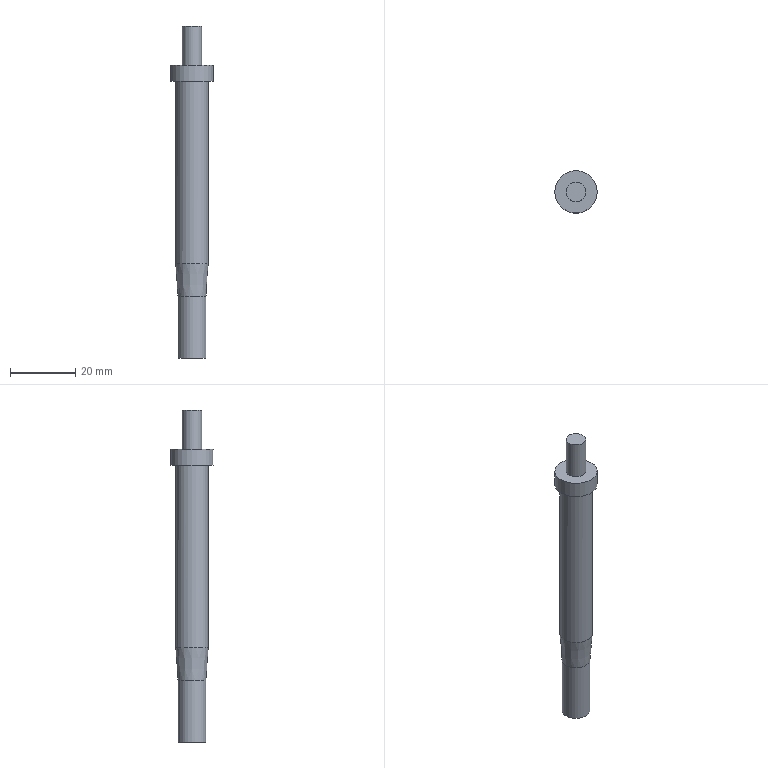Part | NX | features solid 2 | 1 solid | 9 faces | box 13 x 13 x 102 mm | volume 7185 mm3 | plane 4 | cylinder 4 | cone 1 | commonest cylinder face diameters 6 x1 8.6 x1 10 x1 13 x1
STEP:
#1=CARTESIAN_POINT('',(-860.368,-103.697,53.));
#2=VERTEX_POINT('',#1);
#3=CARTESIAN_POINT('',(-864.522,-102.584,53.));
#4=DIRECTION('',(0.,0.,1.));
#5=DIRECTION('',(0.9659,-0.2588,0.));
#6=AXIS2_PLACEMENT_3D('',#3,#4,#5);
#7=CIRCLE('',#6,4.3);
#8=EDGE_CURVE('',#2,#2,#7,.T.);
#9=ORIENTED_EDGE('',*,*,#8,.F.);
#10=EDGE_LOOP('',(#9));
#11=FACE_BOUND('',#10,.T.);
#12=CARTESIAN_POINT('',(-864.522,-102.584,53.));
#13=DIRECTION('',(0.,0.,-1.));
#14=DIRECTION('',(-0.9659,0.2588,0.));
#15=AXIS2_PLACEMENT_3D('',#12,#13,#14);
#16=PLANE('',#15);
#17=ADVANCED_FACE('',(#11),#16,.T.);
#18=CARTESIAN_POINT('',(-860.368,-103.697,72.));
#19=VERTEX_POINT('',#18);
#20=CARTESIAN_POINT('',(-864.522,-102.584,72.));
#21=DIRECTION('',(0.,0.,1.));
#22=DIRECTION('',(0.9659,-0.2588,0.));
#23=AXIS2_PLACEMENT_3D('',#20,#21,#22);
#24=CIRCLE('',#23,4.3);
#25=EDGE_CURVE('',#19,#19,#24,.T.);
#26=ORIENTED_EDGE('',*,*,#25,.F.);
#27=EDGE_LOOP('',(#26));
#28=FACE_BOUND('',#27,.T.);
#29=ORIENTED_EDGE('',*,*,#8,.T.);
#30=EDGE_LOOP('',(#29));
#31=FACE_BOUND('',#30,.T.);
#32=CARTESIAN_POINT('',(-864.522,-102.584,53.));
#33=DIRECTION('',(0.,0.,1.));
#34=DIRECTION('',(0.9659,-0.2588,0.));
#35=AXIS2_PLACEMENT_3D('',#32,#33,#34);
#36=CYLINDRICAL_SURFACE('',#35,4.3);
#37=ADVANCED_FACE('',(#28,#31),#36,.T.);
#38=ORIENTED_EDGE('',*,*,#25,.T.);
#39=EDGE_LOOP('',(#38));
#40=FACE_BOUND('',#39,.T.);
#41=CARTESIAN_POINT('',(-859.692,-103.878,82.));
#42=VERTEX_POINT('',#41);
#43=CARTESIAN_POINT('',(-864.522,-102.584,82.));
#44=DIRECTION('',(0.,0.,1.));
#45=DIRECTION('',(0.9659,-0.2588,0.));
#46=AXIS2_PLACEMENT_3D('',#43,#44,#45);
#47=CIRCLE('',#46,5.);
#48=EDGE_CURVE('',#42,#42,#47,.T.);
#49=ORIENTED_EDGE('',*,*,#48,.F.);
#50=EDGE_LOOP('',(#49));
#51=FACE_BOUND('',#50,.T.);
#52=CARTESIAN_POINT('',(-864.522,-102.584,72.));
#53=DIRECTION('',(0.,0.,1.));
#54=DIRECTION('',(0.9659,-0.2588,0.));
#55=AXIS2_PLACEMENT_3D('',#52,#53,#54);
#56=CONICAL_SURFACE('',#55,4.3,0.06989);
#57=ADVANCED_FACE('',(#40,#51),#56,.T.);
#58=CARTESIAN_POINT('',(-869.522,-102.584,138.));
#59=VERTEX_POINT('',#58);
#60=CARTESIAN_POINT('',(-864.522,-102.584,138.));
#61=DIRECTION('',(0.,0.,-1.));
#62=DIRECTION('',(-1.,0.,0.));
#63=AXIS2_PLACEMENT_3D('',#60,#61,#62);
#64=CIRCLE('',#63,5.);
#65=EDGE_CURVE('',#59,#59,#64,.F.);
#66=ORIENTED_EDGE('',*,*,#65,.F.);
#67=EDGE_LOOP('',(#66));
#68=FACE_BOUND('',#67,.T.);
#69=ORIENTED_EDGE('',*,*,#48,.T.);
#70=EDGE_LOOP('',(#69));
#71=FACE_BOUND('',#70,.T.);
#72=CARTESIAN_POINT('',(-864.522,-102.584,82.));
#73=DIRECTION('',(0.,0.,1.));
#74=DIRECTION('',(0.9659,-0.2588,0.));
#75=AXIS2_PLACEMENT_3D('',#72,#73,#74);
#76=CYLINDRICAL_SURFACE('',#75,5.);
#77=ADVANCED_FACE('',(#68,#71),#76,.T.);
#78=CARTESIAN_POINT('',(-861.522,-102.584,143.));
#79=VERTEX_POINT('',#78);
#80=CARTESIAN_POINT('',(-864.522,-102.584,143.));
#81=DIRECTION('',(0.,0.,1.));
#82=DIRECTION('',(1.,0.,0.));
#83=AXIS2_PLACEMENT_3D('',#80,#81,#82);
#84=CIRCLE('',#83,3.);
#85=EDGE_CURVE('',#79,#79,#84,.T.);
#86=ORIENTED_EDGE('',*,*,#85,.F.);
#87=EDGE_LOOP('',(#86));
#88=FACE_BOUND('',#87,.T.);
#89=CARTESIAN_POINT('',(-858.022,-102.584,143.));
#90=VERTEX_POINT('',#89);
#91=CARTESIAN_POINT('',(-864.522,-102.584,143.));
#92=DIRECTION('',(0.,0.,1.));
#93=DIRECTION('',(1.,0.,0.));
#94=AXIS2_PLACEMENT_3D('',#91,#92,#93);
#95=CIRCLE('',#94,6.5);
#96=EDGE_CURVE('',#90,#90,#95,.F.);
#97=ORIENTED_EDGE('',*,*,#96,.F.);
#98=EDGE_LOOP('',(#97));
#99=FACE_BOUND('',#98,.T.);
#100=CARTESIAN_POINT('',(-864.522,-102.584,143.));
#101=DIRECTION('',(0.,0.,1.));
#102=DIRECTION('',(0.9659,-0.2588,0.));
#103=AXIS2_PLACEMENT_3D('',#100,#101,#102);
#104=PLANE('',#103);
#105=ADVANCED_FACE('',(#88,#99),#104,.T.);
#106=ORIENTED_EDGE('',*,*,#65,.T.);
#107=EDGE_LOOP('',(#106));
#108=FACE_BOUND('',#107,.T.);
#109=CARTESIAN_POINT('',(-871.022,-102.584,138.));
#110=VERTEX_POINT('',#109);
#111=CARTESIAN_POINT('',(-864.522,-102.584,138.));
#112=DIRECTION('',(0.,0.,-1.));
#113=DIRECTION('',(-1.,0.,0.));
#114=AXIS2_PLACEMENT_3D('',#111,#112,#113);
#115=CIRCLE('',#114,6.5);
#116=EDGE_CURVE('',#110,#110,#115,.F.);
#117=ORIENTED_EDGE('',*,*,#116,.F.);
#118=EDGE_LOOP('',(#117));
#119=FACE_BOUND('',#118,.T.);
#120=CARTESIAN_POINT('',(-864.522,-102.584,138.));
#121=DIRECTION('',(0.,0.,-1.));
#122=DIRECTION('',(-0.9659,0.2588,0.));
#123=AXIS2_PLACEMENT_3D('',#120,#121,#122);
#124=PLANE('',#123);
#125=ADVANCED_FACE('',(#108,#119),#124,.T.);
#126=ORIENTED_EDGE('',*,*,#96,.T.);
#127=EDGE_LOOP('',(#126));
#128=FACE_BOUND('',#127,.T.);
#129=ORIENTED_EDGE('',*,*,#116,.T.);
#130=EDGE_LOOP('',(#129));
#131=FACE_BOUND('',#130,.T.);
#132=CARTESIAN_POINT('',(-864.522,-102.584,128.));
#133=DIRECTION('',(0.,0.,1.));
#134=DIRECTION('',(0.9659,-0.2588,0.));
#135=AXIS2_PLACEMENT_3D('',#132,#133,#134);
#136=CYLINDRICAL_SURFACE('',#135,6.5);
#137=ADVANCED_FACE('',(#128,#131),#136,.T.);
#138=CARTESIAN_POINT('',(-861.522,-102.584,155.));
#139=VERTEX_POINT('',#138);
#140=CARTESIAN_POINT('',(-864.522,-102.584,155.));
#141=DIRECTION('',(0.,0.,1.));
#142=DIRECTION('',(1.,0.,0.));
#143=AXIS2_PLACEMENT_3D('',#140,#141,#142);
#144=CIRCLE('',#143,3.);
#145=EDGE_CURVE('',#139,#139,#144,.F.);
#146=ORIENTED_EDGE('',*,*,#145,.F.);
#147=EDGE_LOOP('',(#146));
#148=FACE_BOUND('',#147,.T.);
#149=CARTESIAN_POINT('',(-864.522,-102.584,155.));
#150=DIRECTION('',(0.,0.,1.));
#151=DIRECTION('',(0.9659,-0.2588,0.));
#152=AXIS2_PLACEMENT_3D('',#149,#150,#151);
#153=PLANE('',#152);
#154=ADVANCED_FACE('',(#148),#153,.T.);
#155=ORIENTED_EDGE('',*,*,#145,.T.);
#156=EDGE_LOOP('',(#155));
#157=FACE_BOUND('',#156,.T.);
#158=ORIENTED_EDGE('',*,*,#85,.T.);
#159=EDGE_LOOP('',(#158));
#160=FACE_BOUND('',#159,.T.);
#161=CARTESIAN_POINT('',(-864.522,-102.584,133.));
#162=DIRECTION('',(0.,0.,1.));
#163=DIRECTION('',(0.9659,-0.2588,0.));
#164=AXIS2_PLACEMENT_3D('',#161,#162,#163);
#165=CYLINDRICAL_SURFACE('',#164,3.);
#166=ADVANCED_FACE('',(#157,#160),#165,.T.);
#167=CLOSED_SHELL('',(#17,#37,#57,#77,#105,#125,#137,#154,#166));
#168=MANIFOLD_SOLID_BREP('',#167);
#169=(LENGTH_UNIT()NAMED_UNIT(*)SI_UNIT(.MILLI.,.METRE.));
#170=UNCERTAINTY_MEASURE_WITH_UNIT(LENGTH_MEASURE(0.00001),#169,'','');
#171=(NAMED_UNIT(*)PLANE_ANGLE_UNIT()SI_UNIT($,.RADIAN.));
#172=(NAMED_UNIT(*)SI_UNIT($,.STERADIAN.)SOLID_ANGLE_UNIT());
#173=(GEOMETRIC_REPRESENTATION_CONTEXT(3)GLOBAL_UNCERTAINTY_ASSIGNED_CONTEXT((#170))GLOBAL_UNIT_ASSIGNED_CONTEXT((#169,#171,#172))REPRESENTATION_CONTEXT('',''));
#174=ADVANCED_BREP_SHAPE_REPRESENTATION('',(#168),#173);